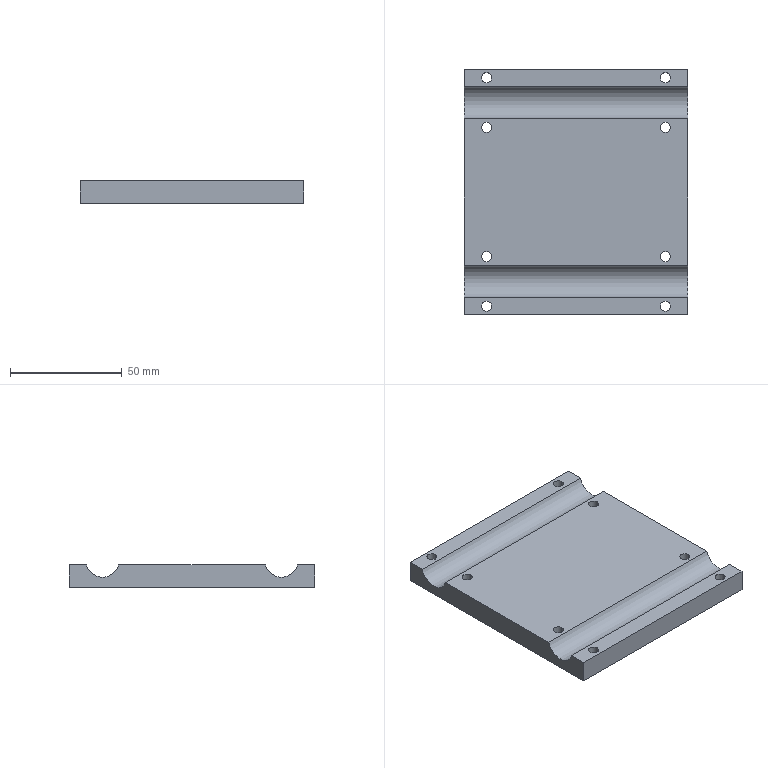Part | STEP file | Cutting module fixing bracket | 1 solid | 26 faces | box 100 x 110 x 10 mm | volume 96984 mm3 | cylinder 18 | plane 8 | commonest cylinder face diameters 4.5 x16 15 x2
STEP:
#1=CARTESIAN_POINT('',(-42.25,68.886,-6.));
#2=VERTEX_POINT('',#1);
#3=CARTESIAN_POINT('',(-37.75,68.886,-6.));
#4=VERTEX_POINT('',#3);
#5=CARTESIAN_POINT('',(-40.,68.886,-6.));
#6=DIRECTION('',(0.,0.,1.));
#7=DIRECTION('',(1.,0.,0.));
#8=AXIS2_PLACEMENT_3D('',#5,#6,#7);
#9=CIRCLE('',#8,2.25);
#10=EDGE_CURVE('',#2,#4,#9,.T.);
#11=ORIENTED_EDGE('',*,*,#10,.F.);
#12=CARTESIAN_POINT('',(-42.25,68.886,4.));
#13=VERTEX_POINT('',#12);
#14=CARTESIAN_POINT('',(-42.25,68.886,-14.));
#15=DIRECTION('',(0.,0.,1.));
#16=VECTOR('',#15,1000.);
#17=LINE('',#14,#16);
#18=EDGE_CURVE('',#2,#13,#17,.T.);
#19=ORIENTED_EDGE('',*,*,#18,.T.);
#20=CARTESIAN_POINT('',(-37.75,68.886,4.));
#21=VERTEX_POINT('',#20);
#22=CARTESIAN_POINT('',(-40.,68.886,4.));
#23=DIRECTION('',(0.,0.,1.));
#24=DIRECTION('',(1.,0.,0.));
#25=AXIS2_PLACEMENT_3D('',#22,#23,#24);
#26=CIRCLE('',#25,2.25);
#27=EDGE_CURVE('',#13,#21,#26,.T.);
#28=ORIENTED_EDGE('',*,*,#27,.T.);
#29=CARTESIAN_POINT('',(-37.75,68.886,-14.));
#30=DIRECTION('',(0.,0.,1.));
#31=VECTOR('',#30,1000.);
#32=LINE('',#29,#31);
#33=EDGE_CURVE('',#4,#21,#32,.T.);
#34=ORIENTED_EDGE('',*,*,#33,.F.);
#35=EDGE_LOOP('',(#11,#19,#28,#34));
#36=FACE_OUTER_BOUND('',#35,.T.);
#37=CARTESIAN_POINT('',(-40.,68.886,-14.));
#38=DIRECTION('',(0.,0.,1.));
#39=DIRECTION('',(1.,0.,0.));
#40=AXIS2_PLACEMENT_3D('',#37,#38,#39);
#41=CYLINDRICAL_SURFACE('',#40,2.25);
#42=ADVANCED_FACE('',(#36),#41,.F.);
#43=CARTESIAN_POINT('',(42.25,68.886,-6.));
#44=VERTEX_POINT('',#43);
#45=CARTESIAN_POINT('',(37.75,68.886,-6.));
#46=VERTEX_POINT('',#45);
#47=CARTESIAN_POINT('',(40.,68.886,-6.));
#48=DIRECTION('',(0.,0.,-1.));
#49=DIRECTION('',(1.,0.,0.));
#50=AXIS2_PLACEMENT_3D('',#47,#48,#49);
#51=CIRCLE('',#50,2.25);
#52=EDGE_CURVE('',#44,#46,#51,.T.);
#53=ORIENTED_EDGE('',*,*,#52,.T.);
#54=CARTESIAN_POINT('',(37.75,68.886,4.));
#55=VERTEX_POINT('',#54);
#56=CARTESIAN_POINT('',(37.75,68.886,-14.));
#57=DIRECTION('',(0.,0.,1.));
#58=VECTOR('',#57,1000.);
#59=LINE('',#56,#58);
#60=EDGE_CURVE('',#46,#55,#59,.T.);
#61=ORIENTED_EDGE('',*,*,#60,.T.);
#62=CARTESIAN_POINT('',(42.25,68.886,4.));
#63=VERTEX_POINT('',#62);
#64=CARTESIAN_POINT('',(40.,68.886,4.));
#65=DIRECTION('',(0.,0.,-1.));
#66=DIRECTION('',(-1.,0.,0.));
#67=AXIS2_PLACEMENT_3D('',#64,#65,#66);
#68=CIRCLE('',#67,2.25);
#69=EDGE_CURVE('',#63,#55,#68,.T.);
#70=ORIENTED_EDGE('',*,*,#69,.F.);
#71=CARTESIAN_POINT('',(42.25,68.886,-14.));
#72=DIRECTION('',(0.,0.,1.));
#73=VECTOR('',#72,1000.);
#74=LINE('',#71,#73);
#75=EDGE_CURVE('',#44,#63,#74,.T.);
#76=ORIENTED_EDGE('',*,*,#75,.F.);
#77=EDGE_LOOP('',(#53,#61,#70,#76));
#78=FACE_OUTER_BOUND('',#77,.T.);
#79=CARTESIAN_POINT('',(40.,68.886,-14.));
#80=DIRECTION('',(0.,0.,1.));
#81=DIRECTION('',(1.,0.,0.));
#82=AXIS2_PLACEMENT_3D('',#79,#80,#81);
#83=CYLINDRICAL_SURFACE('',#82,2.25);
#84=ADVANCED_FACE('',(#78),#83,.F.);
#85=CARTESIAN_POINT('',(37.75,91.114,-6.));
#86=VERTEX_POINT('',#85);
#87=CARTESIAN_POINT('',(42.25,91.114,-6.));
#88=VERTEX_POINT('',#87);
#89=CARTESIAN_POINT('',(40.,91.114,-6.));
#90=DIRECTION('',(0.,0.,1.));
#91=DIRECTION('',(1.,0.,0.));
#92=AXIS2_PLACEMENT_3D('',#89,#90,#91);
#93=CIRCLE('',#92,2.25);
#94=EDGE_CURVE('',#86,#88,#93,.T.);
#95=ORIENTED_EDGE('',*,*,#94,.F.);
#96=CARTESIAN_POINT('',(37.75,91.114,4.));
#97=VERTEX_POINT('',#96);
#98=CARTESIAN_POINT('',(37.75,91.114,-14.));
#99=DIRECTION('',(0.,0.,1.));
#100=VECTOR('',#99,1000.);
#101=LINE('',#98,#100);
#102=EDGE_CURVE('',#86,#97,#101,.T.);
#103=ORIENTED_EDGE('',*,*,#102,.T.);
#104=CARTESIAN_POINT('',(42.25,91.114,4.));
#105=VERTEX_POINT('',#104);
#106=CARTESIAN_POINT('',(40.,91.114,4.));
#107=DIRECTION('',(0.,0.,1.));
#108=DIRECTION('',(-1.,0.,0.));
#109=AXIS2_PLACEMENT_3D('',#106,#107,#108);
#110=CIRCLE('',#109,2.25);
#111=EDGE_CURVE('',#97,#105,#110,.T.);
#112=ORIENTED_EDGE('',*,*,#111,.T.);
#113=CARTESIAN_POINT('',(42.25,91.114,-14.));
#114=DIRECTION('',(0.,0.,1.));
#115=VECTOR('',#114,1000.);
#116=LINE('',#113,#115);
#117=EDGE_CURVE('',#88,#105,#116,.T.);
#118=ORIENTED_EDGE('',*,*,#117,.F.);
#119=EDGE_LOOP('',(#95,#103,#112,#118));
#120=FACE_OUTER_BOUND('',#119,.T.);
#121=CARTESIAN_POINT('',(40.,91.114,-14.));
#122=DIRECTION('',(0.,0.,1.));
#123=DIRECTION('',(1.,0.,0.));
#124=AXIS2_PLACEMENT_3D('',#121,#122,#123);
#125=CYLINDRICAL_SURFACE('',#124,2.25);
#126=ADVANCED_FACE('',(#120),#125,.F.);
#127=CARTESIAN_POINT('',(-37.75,91.114,-6.));
#128=VERTEX_POINT('',#127);
#129=CARTESIAN_POINT('',(-42.25,91.114,-6.));
#130=VERTEX_POINT('',#129);
#131=CARTESIAN_POINT('',(-40.,91.114,-6.));
#132=DIRECTION('',(0.,0.,-1.));
#133=DIRECTION('',(1.,0.,0.));
#134=AXIS2_PLACEMENT_3D('',#131,#132,#133);
#135=CIRCLE('',#134,2.25);
#136=EDGE_CURVE('',#128,#130,#135,.T.);
#137=ORIENTED_EDGE('',*,*,#136,.T.);
#138=CARTESIAN_POINT('',(-42.25,91.114,4.));
#139=VERTEX_POINT('',#138);
#140=CARTESIAN_POINT('',(-42.25,91.114,-14.));
#141=DIRECTION('',(0.,0.,1.));
#142=VECTOR('',#141,1000.);
#143=LINE('',#140,#142);
#144=EDGE_CURVE('',#130,#139,#143,.T.);
#145=ORIENTED_EDGE('',*,*,#144,.T.);
#146=CARTESIAN_POINT('',(-37.75,91.114,4.));
#147=VERTEX_POINT('',#146);
#148=CARTESIAN_POINT('',(-40.,91.114,4.));
#149=DIRECTION('',(0.,0.,-1.));
#150=DIRECTION('',(1.,0.,0.));
#151=AXIS2_PLACEMENT_3D('',#148,#149,#150);
#152=CIRCLE('',#151,2.25);
#153=EDGE_CURVE('',#147,#139,#152,.T.);
#154=ORIENTED_EDGE('',*,*,#153,.F.);
#155=CARTESIAN_POINT('',(-37.75,91.114,-14.));
#156=DIRECTION('',(0.,0.,1.));
#157=VECTOR('',#156,1000.);
#158=LINE('',#155,#157);
#159=EDGE_CURVE('',#128,#147,#158,.T.);
#160=ORIENTED_EDGE('',*,*,#159,.F.);
#161=EDGE_LOOP('',(#137,#145,#154,#160));
#162=FACE_OUTER_BOUND('',#161,.T.);
#163=CARTESIAN_POINT('',(-40.,91.114,-14.));
#164=DIRECTION('',(0.,0.,1.));
#165=DIRECTION('',(1.,0.,0.));
#166=AXIS2_PLACEMENT_3D('',#163,#164,#165);
#167=CYLINDRICAL_SURFACE('',#166,2.25);
#168=ADVANCED_FACE('',(#162),#167,.F.);
#169=CARTESIAN_POINT('',(-37.75,11.114,-6.));
#170=VERTEX_POINT('',#169);
#171=CARTESIAN_POINT('',(-42.25,11.114,-6.));
#172=VERTEX_POINT('',#171);
#173=CARTESIAN_POINT('',(-40.,11.114,-6.));
#174=DIRECTION('',(0.,0.,-1.));
#175=DIRECTION('',(1.,0.,0.));
#176=AXIS2_PLACEMENT_3D('',#173,#174,#175);
#177=CIRCLE('',#176,2.25);
#178=EDGE_CURVE('',#170,#172,#177,.T.);
#179=ORIENTED_EDGE('',*,*,#178,.T.);
#180=CARTESIAN_POINT('',(-42.25,11.114,4.));
#181=VERTEX_POINT('',#180);
#182=CARTESIAN_POINT('',(-42.25,11.114,-14.));
#183=DIRECTION('',(0.,0.,1.));
#184=VECTOR('',#183,1000.);
#185=LINE('',#182,#184);
#186=EDGE_CURVE('',#172,#181,#185,.T.);
#187=ORIENTED_EDGE('',*,*,#186,.T.);
#188=CARTESIAN_POINT('',(-37.75,11.114,4.));
#189=VERTEX_POINT('',#188);
#190=CARTESIAN_POINT('',(-40.,11.114,4.));
#191=DIRECTION('',(0.,0.,-1.));
#192=DIRECTION('',(1.,0.,0.));
#193=AXIS2_PLACEMENT_3D('',#190,#191,#192);
#194=CIRCLE('',#193,2.25);
#195=EDGE_CURVE('',#189,#181,#194,.T.);
#196=ORIENTED_EDGE('',*,*,#195,.F.);
#197=CARTESIAN_POINT('',(-37.75,11.114,-14.));
#198=DIRECTION('',(0.,0.,1.));
#199=VECTOR('',#198,1000.);
#200=LINE('',#197,#199);
#201=EDGE_CURVE('',#170,#189,#200,.T.);
#202=ORIENTED_EDGE('',*,*,#201,.F.);
#203=EDGE_LOOP('',(#179,#187,#196,#202));
#204=FACE_OUTER_BOUND('',#203,.T.);
#205=CARTESIAN_POINT('',(-40.,11.114,-14.));
#206=DIRECTION('',(0.,0.,1.));
#207=DIRECTION('',(1.,0.,0.));
#208=AXIS2_PLACEMENT_3D('',#205,#206,#207);
#209=CYLINDRICAL_SURFACE('',#208,2.25);
#210=ADVANCED_FACE('',(#204),#209,.F.);
#211=CARTESIAN_POINT('',(37.75,11.114,-6.));
#212=VERTEX_POINT('',#211);
#213=CARTESIAN_POINT('',(42.25,11.114,-6.));
#214=VERTEX_POINT('',#213);
#215=CARTESIAN_POINT('',(40.,11.114,-6.));
#216=DIRECTION('',(0.,0.,1.));
#217=DIRECTION('',(1.,0.,0.));
#218=AXIS2_PLACEMENT_3D('',#215,#216,#217);
#219=CIRCLE('',#218,2.25);
#220=EDGE_CURVE('',#212,#214,#219,.T.);
#221=ORIENTED_EDGE('',*,*,#220,.F.);
#222=CARTESIAN_POINT('',(37.75,11.114,4.));
#223=VERTEX_POINT('',#222);
#224=CARTESIAN_POINT('',(37.75,11.114,-14.));
#225=DIRECTION('',(0.,0.,1.));
#226=VECTOR('',#225,1000.);
#227=LINE('',#224,#226);
#228=EDGE_CURVE('',#212,#223,#227,.T.);
#229=ORIENTED_EDGE('',*,*,#228,.T.);
#230=CARTESIAN_POINT('',(42.25,11.114,4.));
#231=VERTEX_POINT('',#230);
#232=CARTESIAN_POINT('',(40.,11.114,4.));
#233=DIRECTION('',(0.,0.,1.));
#234=DIRECTION('',(-1.,0.,0.));
#235=AXIS2_PLACEMENT_3D('',#232,#233,#234);
#236=CIRCLE('',#235,2.25);
#237=EDGE_CURVE('',#223,#231,#236,.T.);
#238=ORIENTED_EDGE('',*,*,#237,.T.);
#239=CARTESIAN_POINT('',(42.25,11.114,-14.));
#240=DIRECTION('',(0.,0.,1.));
#241=VECTOR('',#240,1000.);
#242=LINE('',#239,#241);
#243=EDGE_CURVE('',#214,#231,#242,.T.);
#244=ORIENTED_EDGE('',*,*,#243,.F.);
#245=EDGE_LOOP('',(#221,#229,#238,#244));
#246=FACE_OUTER_BOUND('',#245,.T.);
#247=CARTESIAN_POINT('',(40.,11.114,-14.));
#248=DIRECTION('',(0.,0.,1.));
#249=DIRECTION('',(1.,0.,0.));
#250=AXIS2_PLACEMENT_3D('',#247,#248,#249);
#251=CYLINDRICAL_SURFACE('',#250,2.25);
#252=ADVANCED_FACE('',(#246),#251,.F.);
#253=CARTESIAN_POINT('',(42.25,-11.114,-6.));
#254=VERTEX_POINT('',#253);
#255=CARTESIAN_POINT('',(37.75,-11.114,-6.));
#256=VERTEX_POINT('',#255);
#257=CARTESIAN_POINT('',(40.,-11.114,-6.));
#258=DIRECTION('',(0.,0.,-1.));
#259=DIRECTION('',(1.,0.,0.));
#260=AXIS2_PLACEMENT_3D('',#257,#258,#259);
#261=CIRCLE('',#260,2.25);
#262=EDGE_CURVE('',#254,#256,#261,.T.);
#263=ORIENTED_EDGE('',*,*,#262,.T.);
#264=CARTESIAN_POINT('',(37.75,-11.114,4.));
#265=VERTEX_POINT('',#264);
#266=CARTESIAN_POINT('',(37.75,-11.114,-14.));
#267=DIRECTION('',(0.,0.,1.));
#268=VECTOR('',#267,1000.);
#269=LINE('',#266,#268);
#270=EDGE_CURVE('',#256,#265,#269,.T.);
#271=ORIENTED_EDGE('',*,*,#270,.T.);
#272=CARTESIAN_POINT('',(42.25,-11.114,4.));
#273=VERTEX_POINT('',#272);
#274=CARTESIAN_POINT('',(40.,-11.114,4.));
#275=DIRECTION('',(0.,0.,-1.));
#276=DIRECTION('',(-1.,0.,0.));
#277=AXIS2_PLACEMENT_3D('',#274,#275,#276);
#278=CIRCLE('',#277,2.25);
#279=EDGE_CURVE('',#273,#265,#278,.T.);
#280=ORIENTED_EDGE('',*,*,#279,.F.);
#281=CARTESIAN_POINT('',(42.25,-11.114,-14.));
#282=DIRECTION('',(0.,0.,1.));
#283=VECTOR('',#282,1000.);
#284=LINE('',#281,#283);
#285=EDGE_CURVE('',#254,#273,#284,.T.);
#286=ORIENTED_EDGE('',*,*,#285,.F.);
#287=EDGE_LOOP('',(#263,#271,#280,#286));
#288=FACE_OUTER_BOUND('',#287,.T.);
#289=CARTESIAN_POINT('',(40.,-11.114,-14.));
#290=DIRECTION('',(0.,0.,1.));
#291=DIRECTION('',(1.,0.,0.));
#292=AXIS2_PLACEMENT_3D('',#289,#290,#291);
#293=CYLINDRICAL_SURFACE('',#292,2.25);
#294=ADVANCED_FACE('',(#288),#293,.F.);
#295=CARTESIAN_POINT('',(-42.25,-11.114,-6.));
#296=VERTEX_POINT('',#295);
#297=CARTESIAN_POINT('',(-37.75,-11.114,-6.));
#298=VERTEX_POINT('',#297);
#299=CARTESIAN_POINT('',(-40.,-11.114,-6.));
#300=DIRECTION('',(0.,0.,1.));
#301=DIRECTION('',(1.,0.,0.));
#302=AXIS2_PLACEMENT_3D('',#299,#300,#301);
#303=CIRCLE('',#302,2.25);
#304=EDGE_CURVE('',#296,#298,#303,.T.);
#305=ORIENTED_EDGE('',*,*,#304,.F.);
#306=CARTESIAN_POINT('',(-42.25,-11.114,4.));
#307=VERTEX_POINT('',#306);
#308=CARTESIAN_POINT('',(-42.25,-11.114,-14.));
#309=DIRECTION('',(0.,0.,1.));
#310=VECTOR('',#309,1000.);
#311=LINE('',#308,#310);
#312=EDGE_CURVE('',#296,#307,#311,.T.);
#313=ORIENTED_EDGE('',*,*,#312,.T.);
#314=CARTESIAN_POINT('',(-37.75,-11.114,4.));
#315=VERTEX_POINT('',#314);
#316=CARTESIAN_POINT('',(-40.,-11.114,4.));
#317=DIRECTION('',(0.,0.,1.));
#318=DIRECTION('',(1.,0.,0.));
#319=AXIS2_PLACEMENT_3D('',#316,#317,#318);
#320=CIRCLE('',#319,2.25);
#321=EDGE_CURVE('',#307,#315,#320,.T.);
#322=ORIENTED_EDGE('',*,*,#321,.T.);
#323=CARTESIAN_POINT('',(-37.75,-11.114,-14.));
#324=DIRECTION('',(0.,0.,1.));
#325=VECTOR('',#324,1000.);
#326=LINE('',#323,#325);
#327=EDGE_CURVE('',#298,#315,#326,.T.);
#328=ORIENTED_EDGE('',*,*,#327,.F.);
#329=EDGE_LOOP('',(#305,#313,#322,#328));
#330=FACE_OUTER_BOUND('',#329,.T.);
#331=CARTESIAN_POINT('',(-40.,-11.114,-14.));
#332=DIRECTION('',(0.,0.,1.));
#333=DIRECTION('',(1.,0.,0.));
#334=AXIS2_PLACEMENT_3D('',#331,#332,#333);
#335=CYLINDRICAL_SURFACE('',#334,2.25);
#336=ADVANCED_FACE('',(#330),#335,.F.);
#337=CARTESIAN_POINT('',(-40.,68.886,4.));
#338=DIRECTION('',(0.,0.,1.));
#339=DIRECTION('',(1.,0.,0.));
#340=AXIS2_PLACEMENT_3D('',#337,#338,#339);
#341=CIRCLE('',#340,2.25);
#342=EDGE_CURVE('',#21,#13,#341,.T.);
#343=ORIENTED_EDGE('',*,*,#342,.F.);
#344=ORIENTED_EDGE('',*,*,#27,.F.);
#345=EDGE_LOOP('',(#343,#344));
#346=FACE_BOUND('',#345,.T.);
#347=ORIENTED_EDGE('',*,*,#69,.T.);
#348=CARTESIAN_POINT('',(40.,68.886,4.));
#349=DIRECTION('',(0.,0.,-1.));
#350=DIRECTION('',(-1.,0.,0.));
#351=AXIS2_PLACEMENT_3D('',#348,#349,#350);
#352=CIRCLE('',#351,2.25);
#353=EDGE_CURVE('',#55,#63,#352,.T.);
#354=ORIENTED_EDGE('',*,*,#353,.T.);
#355=EDGE_LOOP('',(#347,#354));
#356=FACE_BOUND('',#355,.T.);
#357=CARTESIAN_POINT('',(40.,11.114,4.));
#358=DIRECTION('',(0.,0.,1.));
#359=DIRECTION('',(-1.,0.,0.));
#360=AXIS2_PLACEMENT_3D('',#357,#358,#359);
#361=CIRCLE('',#360,2.25);
#362=EDGE_CURVE('',#231,#223,#361,.T.);
#363=ORIENTED_EDGE('',*,*,#362,.F.);
#364=ORIENTED_EDGE('',*,*,#237,.F.);
#365=EDGE_LOOP('',(#363,#364));
#366=FACE_BOUND('',#365,.T.);
#367=ORIENTED_EDGE('',*,*,#195,.T.);
#368=CARTESIAN_POINT('',(-40.,11.114,4.));
#369=DIRECTION('',(0.,0.,-1.));
#370=DIRECTION('',(1.,0.,0.));
#371=AXIS2_PLACEMENT_3D('',#368,#369,#370);
#372=CIRCLE('',#371,2.25);
#373=EDGE_CURVE('',#181,#189,#372,.T.);
#374=ORIENTED_EDGE('',*,*,#373,.T.);
#375=EDGE_LOOP('',(#367,#374));
#376=FACE_BOUND('',#375,.T.);
#377=CARTESIAN_POINT('',(-50.,72.772,4.));
#378=VERTEX_POINT('',#377);
#379=CARTESIAN_POINT('',(50.,72.772,4.));
#380=VERTEX_POINT('',#379);
#381=CARTESIAN_POINT('',(66.,72.772,4.));
#382=DIRECTION('',(1.,0.,0.));
#383=VECTOR('',#382,1000.);
#384=LINE('',#381,#383);
#385=EDGE_CURVE('',#378,#380,#384,.T.);
#386=ORIENTED_EDGE('',*,*,#385,.F.);
#387=CARTESIAN_POINT('',(-50.,7.228,4.));
#388=VERTEX_POINT('',#387);
#389=CARTESIAN_POINT('',(-50.,-15.,4.));
#390=DIRECTION('',(0.,-1.,0.));
#391=VECTOR('',#390,1000.);
#392=LINE('',#389,#391);
#393=EDGE_CURVE('',#378,#388,#392,.T.);
#394=ORIENTED_EDGE('',*,*,#393,.T.);
#395=CARTESIAN_POINT('',(50.,7.228,4.));
#396=VERTEX_POINT('',#395);
#397=CARTESIAN_POINT('',(66.,7.228,4.));
#398=DIRECTION('',(-1.,0.,0.));
#399=VECTOR('',#398,1000.);
#400=LINE('',#397,#399);
#401=EDGE_CURVE('',#396,#388,#400,.T.);
#402=ORIENTED_EDGE('',*,*,#401,.F.);
#403=CARTESIAN_POINT('',(50.,15.,4.));
#404=DIRECTION('',(0.,-1.,0.));
#405=VECTOR('',#404,1000.);
#406=LINE('',#403,#405);
#407=EDGE_CURVE('',#380,#396,#406,.T.);
#408=ORIENTED_EDGE('',*,*,#407,.F.);
#409=EDGE_LOOP('',(#386,#394,#402,#408));
#410=FACE_OUTER_BOUND('',#409,.T.);
#411=CARTESIAN_POINT('',(0.,0.,4.));
#412=DIRECTION('',(0.,0.,-1.));
#413=DIRECTION('',(-1.,0.,0.));
#414=AXIS2_PLACEMENT_3D('',#411,#412,#413);
#415=PLANE('',#414);
#416=ADVANCED_FACE('',(#346,#356,#366,#376,#410),#415,.F.);
#417=CARTESIAN_POINT('',(40.,91.114,4.));
#418=DIRECTION('',(0.,0.,1.));
#419=DIRECTION('',(-1.,0.,0.));
#420=AXIS2_PLACEMENT_3D('',#417,#418,#419);
#421=CIRCLE('',#420,2.25);
#422=EDGE_CURVE('',#105,#97,#421,.T.);
#423=ORIENTED_EDGE('',*,*,#422,.F.);
#424=ORIENTED_EDGE('',*,*,#111,.F.);
#425=EDGE_LOOP('',(#423,#424));
#426=FACE_BOUND('',#425,.T.);
#427=ORIENTED_EDGE('',*,*,#153,.T.);
#428=CARTESIAN_POINT('',(-40.,91.114,4.));
#429=DIRECTION('',(0.,0.,-1.));
#430=DIRECTION('',(1.,0.,0.));
#431=AXIS2_PLACEMENT_3D('',#428,#429,#430);
#432=CIRCLE('',#431,2.25);
#433=EDGE_CURVE('',#139,#147,#432,.T.);
#434=ORIENTED_EDGE('',*,*,#433,.T.);
#435=EDGE_LOOP('',(#427,#434));
#436=FACE_BOUND('',#435,.T.);
#437=CARTESIAN_POINT('',(50.,87.228,4.));
#438=VERTEX_POINT('',#437);
#439=CARTESIAN_POINT('',(-50.,87.228,4.));
#440=VERTEX_POINT('',#439);
#441=CARTESIAN_POINT('',(66.,87.228,4.));
#442=DIRECTION('',(-1.,0.,0.));
#443=VECTOR('',#442,1000.);
#444=LINE('',#441,#443);
#445=EDGE_CURVE('',#438,#440,#444,.T.);
#446=ORIENTED_EDGE('',*,*,#445,.F.);
#447=CARTESIAN_POINT('',(50.,95.,4.));
#448=VERTEX_POINT('',#447);
#449=CARTESIAN_POINT('',(50.,15.,4.));
#450=DIRECTION('',(0.,-1.,0.));
#451=VECTOR('',#450,1000.);
#452=LINE('',#449,#451);
#453=EDGE_CURVE('',#448,#438,#452,.T.);
#454=ORIENTED_EDGE('',*,*,#453,.F.);
#455=CARTESIAN_POINT('',(-50.,95.,4.));
#456=VERTEX_POINT('',#455);
#457=CARTESIAN_POINT('',(-50.,95.,4.));
#458=DIRECTION('',(1.,0.,0.));
#459=VECTOR('',#458,1000.);
#460=LINE('',#457,#459);
#461=EDGE_CURVE('',#456,#448,#460,.T.);
#462=ORIENTED_EDGE('',*,*,#461,.F.);
#463=CARTESIAN_POINT('',(-50.,-15.,4.));
#464=DIRECTION('',(0.,-1.,0.));
#465=VECTOR('',#464,1000.);
#466=LINE('',#463,#465);
#467=EDGE_CURVE('',#456,#440,#466,.T.);
#468=ORIENTED_EDGE('',*,*,#467,.T.);
#469=EDGE_LOOP('',(#446,#454,#462,#468));
#470=FACE_OUTER_BOUND('',#469,.T.);
#471=CARTESIAN_POINT('',(0.,0.,4.));
#472=DIRECTION('',(0.,0.,-1.));
#473=DIRECTION('',(-1.,0.,0.));
#474=AXIS2_PLACEMENT_3D('',#471,#472,#473);
#475=PLANE('',#474);
#476=ADVANCED_FACE('',(#426,#436,#470),#475,.F.);
#477=CARTESIAN_POINT('',(50.,80.,6.));
#478=DIRECTION('',(1.,0.,0.));
#479=DIRECTION('',(0.,0.,1.));
#480=AXIS2_PLACEMENT_3D('',#477,#478,#479);
#481=CIRCLE('',#480,7.5);
#482=EDGE_CURVE('',#380,#438,#481,.T.);
#483=ORIENTED_EDGE('',*,*,#482,.F.);
#484=ORIENTED_EDGE('',*,*,#407,.T.);
#485=CARTESIAN_POINT('',(50.,-7.228,4.));
#486=VERTEX_POINT('',#485);
#487=CARTESIAN_POINT('',(50.,0.,6.));
#488=DIRECTION('',(-1.,0.,0.));
#489=DIRECTION('',(0.,0.,1.));
#490=AXIS2_PLACEMENT_3D('',#487,#488,#489);
#491=CIRCLE('',#490,7.5);
#492=EDGE_CURVE('',#396,#486,#491,.T.);
#493=ORIENTED_EDGE('',*,*,#492,.T.);
#494=CARTESIAN_POINT('',(50.,-15.,4.));
#495=VERTEX_POINT('',#494);
#496=CARTESIAN_POINT('',(50.,15.,4.));
#497=DIRECTION('',(0.,-1.,0.));
#498=VECTOR('',#497,1000.);
#499=LINE('',#496,#498);
#500=EDGE_CURVE('',#486,#495,#499,.T.);
#501=ORIENTED_EDGE('',*,*,#500,.T.);
#502=CARTESIAN_POINT('',(50.,-15.,-6.));
#503=VERTEX_POINT('',#502);
#504=CARTESIAN_POINT('',(50.,-15.,6.));
#505=DIRECTION('',(0.,0.,-1.));
#506=VECTOR('',#505,1000.);
#507=LINE('',#504,#506);
#508=EDGE_CURVE('',#495,#503,#507,.T.);
#509=ORIENTED_EDGE('',*,*,#508,.T.);
#510=CARTESIAN_POINT('',(50.,95.,-6.));
#511=VERTEX_POINT('',#510);
#512=CARTESIAN_POINT('',(50.,15.,-6.));
#513=DIRECTION('',(0.,1.,0.));
#514=VECTOR('',#513,1000.);
#515=LINE('',#512,#514);
#516=EDGE_CURVE('',#503,#511,#515,.T.);
#517=ORIENTED_EDGE('',*,*,#516,.T.);
#518=CARTESIAN_POINT('',(50.,95.,4.));
#519=DIRECTION('',(0.,0.,-1.));
#520=VECTOR('',#519,1000.);
#521=LINE('',#518,#520);
#522=EDGE_CURVE('',#448,#511,#521,.T.);
#523=ORIENTED_EDGE('',*,*,#522,.F.);
#524=ORIENTED_EDGE('',*,*,#453,.T.);
#525=EDGE_LOOP('',(#483,#484,#493,#501,#509,#517,#523,#524));
#526=FACE_OUTER_BOUND('',#525,.T.);
#527=CARTESIAN_POINT('',(50.,15.,6.));
#528=DIRECTION('',(-1.,0.,0.));
#529=DIRECTION('',(0.,0.,1.));
#530=AXIS2_PLACEMENT_3D('',#527,#528,#529);
#531=PLANE('',#530);
#532=ADVANCED_FACE('',(#526),#531,.F.);
#533=CARTESIAN_POINT('',(-50.,80.,6.));
#534=DIRECTION('',(1.,0.,0.));
#535=DIRECTION('',(0.,1.,0.));
#536=AXIS2_PLACEMENT_3D('',#533,#534,#535);
#537=CIRCLE('',#536,7.5);
#538=EDGE_CURVE('',#378,#440,#537,.T.);
#539=ORIENTED_EDGE('',*,*,#538,.T.);
#540=ORIENTED_EDGE('',*,*,#467,.F.);
#541=CARTESIAN_POINT('',(-50.,95.,-6.));
#542=VERTEX_POINT('',#541);
#543=CARTESIAN_POINT('',(-50.,95.,-6.));
#544=DIRECTION('',(0.,0.,1.));
#545=VECTOR('',#544,1000.);
#546=LINE('',#543,#545);
#547=EDGE_CURVE('',#542,#456,#546,.T.);
#548=ORIENTED_EDGE('',*,*,#547,.F.);
#549=CARTESIAN_POINT('',(-50.,-15.,-6.));
#550=VERTEX_POINT('',#549);
#551=CARTESIAN_POINT('',(-50.,15.,-6.));
#552=DIRECTION('',(0.,-1.,0.));
#553=VECTOR('',#552,1000.);
#554=LINE('',#551,#553);
#555=EDGE_CURVE('',#542,#550,#554,.T.);
#556=ORIENTED_EDGE('',*,*,#555,.T.);
#557=CARTESIAN_POINT('',(-50.,-15.,4.));
#558=VERTEX_POINT('',#557);
#559=CARTESIAN_POINT('',(-50.,-15.,6.));
#560=DIRECTION('',(0.,0.,-1.));
#561=VECTOR('',#560,1000.);
#562=LINE('',#559,#561);
#563=EDGE_CURVE('',#558,#550,#562,.T.);
#564=ORIENTED_EDGE('',*,*,#563,.F.);
#565=CARTESIAN_POINT('',(-50.,-7.228,4.));
#566=VERTEX_POINT('',#565);
#567=CARTESIAN_POINT('',(-50.,-15.,4.));
#568=DIRECTION('',(0.,-1.,0.));
#569=VECTOR('',#568,1000.);
#570=LINE('',#567,#569);
#571=EDGE_CURVE('',#566,#558,#570,.T.);
#572=ORIENTED_EDGE('',*,*,#571,.F.);
#573=CARTESIAN_POINT('',(-50.,0.,6.));
#574=DIRECTION('',(-1.,0.,0.));
#575=DIRECTION('',(0.,-1.,0.));
#576=AXIS2_PLACEMENT_3D('',#573,#574,#575);
#577=CIRCLE('',#576,7.5);
#578=EDGE_CURVE('',#388,#566,#577,.T.);
#579=ORIENTED_EDGE('',*,*,#578,.F.);
#580=ORIENTED_EDGE('',*,*,#393,.F.);
#581=EDGE_LOOP('',(#539,#540,#548,#556,#564,#572,#579,#580));
#582=FACE_OUTER_BOUND('',#581,.T.);
#583=CARTESIAN_POINT('',(-50.,15.,6.));
#584=DIRECTION('',(1.,0.,0.));
#585=DIRECTION('',(0.,0.,-1.));
#586=AXIS2_PLACEMENT_3D('',#583,#584,#585);
#587=PLANE('',#586);
#588=ADVANCED_FACE('',(#582),#587,.F.);
#589=ORIENTED_EDGE('',*,*,#508,.F.);
#590=CARTESIAN_POINT('',(-50.,-15.,4.));
#591=DIRECTION('',(1.,0.,0.));
#592=VECTOR('',#591,1000.);
#593=LINE('',#590,#592);
#594=EDGE_CURVE('',#558,#495,#593,.T.);
#595=ORIENTED_EDGE('',*,*,#594,.F.);
#596=ORIENTED_EDGE('',*,*,#563,.T.);
#597=CARTESIAN_POINT('',(-50.,-15.,-6.));
#598=DIRECTION('',(1.,0.,0.));
#599=VECTOR('',#598,1000.);
#600=LINE('',#597,#599);
#601=EDGE_CURVE('',#550,#503,#600,.T.);
#602=ORIENTED_EDGE('',*,*,#601,.T.);
#603=EDGE_LOOP('',(#589,#595,#596,#602));
#604=FACE_OUTER_BOUND('',#603,.T.);
#605=CARTESIAN_POINT('',(-50.,-15.,6.));
#606=DIRECTION('',(0.,1.,0.));
#607=DIRECTION('',(0.,0.,1.));
#608=AXIS2_PLACEMENT_3D('',#605,#606,#607);
#609=PLANE('',#608);
#610=ADVANCED_FACE('',(#604),#609,.F.);
#611=CARTESIAN_POINT('',(-40.,68.886,-6.));
#612=DIRECTION('',(0.,0.,1.));
#613=DIRECTION('',(1.,0.,0.));
#614=AXIS2_PLACEMENT_3D('',#611,#612,#613);
#615=CIRCLE('',#614,2.25);
#616=EDGE_CURVE('',#4,#2,#615,.T.);
#617=ORIENTED_EDGE('',*,*,#616,.T.);
#618=ORIENTED_EDGE('',*,*,#10,.T.);
#619=EDGE_LOOP('',(#617,#618));
#620=FACE_BOUND('',#619,.T.);
#621=ORIENTED_EDGE('',*,*,#52,.F.);
#622=CARTESIAN_POINT('',(40.,68.886,-6.));
#623=DIRECTION('',(0.,0.,-1.));
#624=DIRECTION('',(1.,0.,0.));
#625=AXIS2_PLACEMENT_3D('',#622,#623,#624);
#626=CIRCLE('',#625,2.25);
#627=EDGE_CURVE('',#46,#44,#626,.T.);
#628=ORIENTED_EDGE('',*,*,#627,.F.);
#629=EDGE_LOOP('',(#621,#628));
#630=FACE_BOUND('',#629,.T.);
#631=CARTESIAN_POINT('',(40.,91.114,-6.));
#632=DIRECTION('',(0.,0.,1.));
#633=DIRECTION('',(1.,0.,0.));
#634=AXIS2_PLACEMENT_3D('',#631,#632,#633);
#635=CIRCLE('',#634,2.25);
#636=EDGE_CURVE('',#88,#86,#635,.T.);
#637=ORIENTED_EDGE('',*,*,#636,.T.);
#638=ORIENTED_EDGE('',*,*,#94,.T.);
#639=EDGE_LOOP('',(#637,#638));
#640=FACE_BOUND('',#639,.T.);
#641=ORIENTED_EDGE('',*,*,#136,.F.);
#642=CARTESIAN_POINT('',(-40.,91.114,-6.));
#643=DIRECTION('',(0.,0.,-1.));
#644=DIRECTION('',(1.,0.,0.));
#645=AXIS2_PLACEMENT_3D('',#642,#643,#644);
#646=CIRCLE('',#645,2.25);
#647=EDGE_CURVE('',#130,#128,#646,.T.);
#648=ORIENTED_EDGE('',*,*,#647,.F.);
#649=EDGE_LOOP('',(#641,#648));
#650=FACE_BOUND('',#649,.T.);
#651=ORIENTED_EDGE('',*,*,#178,.F.);
#652=CARTESIAN_POINT('',(-40.,11.114,-6.));
#653=DIRECTION('',(0.,0.,-1.));
#654=DIRECTION('',(1.,0.,0.));
#655=AXIS2_PLACEMENT_3D('',#652,#653,#654);
#656=CIRCLE('',#655,2.25);
#657=EDGE_CURVE('',#172,#170,#656,.T.);
#658=ORIENTED_EDGE('',*,*,#657,.F.);
#659=EDGE_LOOP('',(#651,#658));
#660=FACE_BOUND('',#659,.T.);
#661=CARTESIAN_POINT('',(40.,11.114,-6.));
#662=DIRECTION('',(0.,0.,1.));
#663=DIRECTION('',(1.,0.,0.));
#664=AXIS2_PLACEMENT_3D('',#661,#662,#663);
#665=CIRCLE('',#664,2.25);
#666=EDGE_CURVE('',#214,#212,#665,.T.);
#667=ORIENTED_EDGE('',*,*,#666,.T.);
#668=ORIENTED_EDGE('',*,*,#220,.T.);
#669=EDGE_LOOP('',(#667,#668));
#670=FACE_BOUND('',#669,.T.);
#671=ORIENTED_EDGE('',*,*,#262,.F.);
#672=CARTESIAN_POINT('',(40.,-11.114,-6.));
#673=DIRECTION('',(0.,0.,-1.));
#674=DIRECTION('',(1.,0.,0.));
#675=AXIS2_PLACEMENT_3D('',#672,#673,#674);
#676=CIRCLE('',#675,2.25);
#677=EDGE_CURVE('',#256,#254,#676,.T.);
#678=ORIENTED_EDGE('',*,*,#677,.F.);
#679=EDGE_LOOP('',(#671,#678));
#680=FACE_BOUND('',#679,.T.);
#681=CARTESIAN_POINT('',(-40.,-11.114,-6.));
#682=DIRECTION('',(0.,0.,1.));
#683=DIRECTION('',(1.,0.,0.));
#684=AXIS2_PLACEMENT_3D('',#681,#682,#683);
#685=CIRCLE('',#684,2.25);
#686=EDGE_CURVE('',#298,#296,#685,.T.);
#687=ORIENTED_EDGE('',*,*,#686,.T.);
#688=ORIENTED_EDGE('',*,*,#304,.T.);
#689=EDGE_LOOP('',(#687,#688));
#690=FACE_BOUND('',#689,.T.);
#691=ORIENTED_EDGE('',*,*,#516,.F.);
#692=ORIENTED_EDGE('',*,*,#601,.F.);
#693=ORIENTED_EDGE('',*,*,#555,.F.);
#694=CARTESIAN_POINT('',(50.,95.,-6.));
#695=DIRECTION('',(-1.,0.,0.));
#696=VECTOR('',#695,1000.);
#697=LINE('',#694,#696);
#698=EDGE_CURVE('',#511,#542,#697,.T.);
#699=ORIENTED_EDGE('',*,*,#698,.F.);
#700=EDGE_LOOP('',(#691,#692,#693,#699));
#701=FACE_OUTER_BOUND('',#700,.T.);
#702=CARTESIAN_POINT('',(0.,0.,-6.));
#703=DIRECTION('',(0.,0.,1.));
#704=DIRECTION('',(1.,0.,0.));
#705=AXIS2_PLACEMENT_3D('',#702,#703,#704);
#706=PLANE('',#705);
#707=ADVANCED_FACE('',(#620,#630,#640,#650,#660,#670,#680,#690,#701),#706,.F.);
#708=ORIENTED_EDGE('',*,*,#578,.T.);
#709=CARTESIAN_POINT('',(66.,-7.228,4.));
#710=DIRECTION('',(1.,0.,0.));
#711=VECTOR('',#710,1000.);
#712=LINE('',#709,#711);
#713=EDGE_CURVE('',#566,#486,#712,.T.);
#714=ORIENTED_EDGE('',*,*,#713,.T.);
#715=ORIENTED_EDGE('',*,*,#492,.F.);
#716=ORIENTED_EDGE('',*,*,#401,.T.);
#717=EDGE_LOOP('',(#708,#714,#715,#716));
#718=FACE_OUTER_BOUND('',#717,.T.);
#719=CARTESIAN_POINT('',(66.,0.,6.));
#720=DIRECTION('',(-1.,0.,0.));
#721=DIRECTION('',(0.,-1.,0.));
#722=AXIS2_PLACEMENT_3D('',#719,#720,#721);
#723=CYLINDRICAL_SURFACE('',#722,7.5);
#724=ADVANCED_FACE('',(#718),#723,.F.);
#725=ORIENTED_EDGE('',*,*,#279,.T.);
#726=CARTESIAN_POINT('',(40.,-11.114,4.));
#727=DIRECTION('',(0.,0.,-1.));
#728=DIRECTION('',(-1.,0.,0.));
#729=AXIS2_PLACEMENT_3D('',#726,#727,#728);
#730=CIRCLE('',#729,2.25);
#731=EDGE_CURVE('',#265,#273,#730,.T.);
#732=ORIENTED_EDGE('',*,*,#731,.T.);
#733=EDGE_LOOP('',(#725,#732));
#734=FACE_BOUND('',#733,.T.);
#735=CARTESIAN_POINT('',(-40.,-11.114,4.));
#736=DIRECTION('',(0.,0.,1.));
#737=DIRECTION('',(1.,0.,0.));
#738=AXIS2_PLACEMENT_3D('',#735,#736,#737);
#739=CIRCLE('',#738,2.25);
#740=EDGE_CURVE('',#315,#307,#739,.T.);
#741=ORIENTED_EDGE('',*,*,#740,.F.);
#742=ORIENTED_EDGE('',*,*,#321,.F.);
#743=EDGE_LOOP('',(#741,#742));
#744=FACE_BOUND('',#743,.T.);
#745=ORIENTED_EDGE('',*,*,#713,.F.);
#746=ORIENTED_EDGE('',*,*,#571,.T.);
#747=ORIENTED_EDGE('',*,*,#594,.T.);
#748=ORIENTED_EDGE('',*,*,#500,.F.);
#749=EDGE_LOOP('',(#745,#746,#747,#748));
#750=FACE_OUTER_BOUND('',#749,.T.);
#751=CARTESIAN_POINT('',(0.,0.,4.));
#752=DIRECTION('',(0.,0.,-1.));
#753=DIRECTION('',(-1.,0.,0.));
#754=AXIS2_PLACEMENT_3D('',#751,#752,#753);
#755=PLANE('',#754);
#756=ADVANCED_FACE('',(#734,#744,#750),#755,.F.);
#757=ORIENTED_EDGE('',*,*,#312,.F.);
#758=ORIENTED_EDGE('',*,*,#686,.F.);
#759=ORIENTED_EDGE('',*,*,#327,.T.);
#760=ORIENTED_EDGE('',*,*,#740,.T.);
#761=EDGE_LOOP('',(#757,#758,#759,#760));
#762=FACE_OUTER_BOUND('',#761,.T.);
#763=CARTESIAN_POINT('',(-40.,-11.114,-14.));
#764=DIRECTION('',(0.,0.,1.));
#765=DIRECTION('',(1.,0.,0.));
#766=AXIS2_PLACEMENT_3D('',#763,#764,#765);
#767=CYLINDRICAL_SURFACE('',#766,2.25);
#768=ADVANCED_FACE('',(#762),#767,.F.);
#769=ORIENTED_EDGE('',*,*,#270,.F.);
#770=ORIENTED_EDGE('',*,*,#677,.T.);
#771=ORIENTED_EDGE('',*,*,#285,.T.);
#772=ORIENTED_EDGE('',*,*,#731,.F.);
#773=EDGE_LOOP('',(#769,#770,#771,#772));
#774=FACE_OUTER_BOUND('',#773,.T.);
#775=CARTESIAN_POINT('',(40.,-11.114,-14.));
#776=DIRECTION('',(0.,0.,1.));
#777=DIRECTION('',(1.,0.,0.));
#778=AXIS2_PLACEMENT_3D('',#775,#776,#777);
#779=CYLINDRICAL_SURFACE('',#778,2.25);
#780=ADVANCED_FACE('',(#774),#779,.F.);
#781=ORIENTED_EDGE('',*,*,#228,.F.);
#782=ORIENTED_EDGE('',*,*,#666,.F.);
#783=ORIENTED_EDGE('',*,*,#243,.T.);
#784=ORIENTED_EDGE('',*,*,#362,.T.);
#785=EDGE_LOOP('',(#781,#782,#783,#784));
#786=FACE_OUTER_BOUND('',#785,.T.);
#787=CARTESIAN_POINT('',(40.,11.114,-14.));
#788=DIRECTION('',(0.,0.,1.));
#789=DIRECTION('',(1.,0.,0.));
#790=AXIS2_PLACEMENT_3D('',#787,#788,#789);
#791=CYLINDRICAL_SURFACE('',#790,2.25);
#792=ADVANCED_FACE('',(#786),#791,.F.);
#793=ORIENTED_EDGE('',*,*,#186,.F.);
#794=ORIENTED_EDGE('',*,*,#657,.T.);
#795=ORIENTED_EDGE('',*,*,#201,.T.);
#796=ORIENTED_EDGE('',*,*,#373,.F.);
#797=EDGE_LOOP('',(#793,#794,#795,#796));
#798=FACE_OUTER_BOUND('',#797,.T.);
#799=CARTESIAN_POINT('',(-40.,11.114,-14.));
#800=DIRECTION('',(0.,0.,1.));
#801=DIRECTION('',(1.,0.,0.));
#802=AXIS2_PLACEMENT_3D('',#799,#800,#801);
#803=CYLINDRICAL_SURFACE('',#802,2.25);
#804=ADVANCED_FACE('',(#798),#803,.F.);
#805=ORIENTED_EDGE('',*,*,#698,.T.);
#806=ORIENTED_EDGE('',*,*,#547,.T.);
#807=ORIENTED_EDGE('',*,*,#461,.T.);
#808=ORIENTED_EDGE('',*,*,#522,.T.);
#809=EDGE_LOOP('',(#805,#806,#807,#808));
#810=FACE_OUTER_BOUND('',#809,.T.);
#811=CARTESIAN_POINT('',(0.,95.,0.));
#812=DIRECTION('',(0.,1.,0.));
#813=DIRECTION('',(0.,0.,1.));
#814=AXIS2_PLACEMENT_3D('',#811,#812,#813);
#815=PLANE('',#814);
#816=ADVANCED_FACE('',(#810),#815,.T.);
#817=ORIENTED_EDGE('',*,*,#385,.T.);
#818=ORIENTED_EDGE('',*,*,#482,.T.);
#819=ORIENTED_EDGE('',*,*,#445,.T.);
#820=ORIENTED_EDGE('',*,*,#538,.F.);
#821=EDGE_LOOP('',(#817,#818,#819,#820));
#822=FACE_OUTER_BOUND('',#821,.T.);
#823=CARTESIAN_POINT('',(66.,80.,6.));
#824=DIRECTION('',(-1.,0.,0.));
#825=DIRECTION('',(0.,-1.,0.));
#826=AXIS2_PLACEMENT_3D('',#823,#824,#825);
#827=CYLINDRICAL_SURFACE('',#826,7.5);
#828=ADVANCED_FACE('',(#822),#827,.F.);
#829=ORIENTED_EDGE('',*,*,#144,.F.);
#830=ORIENTED_EDGE('',*,*,#647,.T.);
#831=ORIENTED_EDGE('',*,*,#159,.T.);
#832=ORIENTED_EDGE('',*,*,#433,.F.);
#833=EDGE_LOOP('',(#829,#830,#831,#832));
#834=FACE_OUTER_BOUND('',#833,.T.);
#835=CARTESIAN_POINT('',(-40.,91.114,-14.));
#836=DIRECTION('',(0.,0.,1.));
#837=DIRECTION('',(1.,0.,0.));
#838=AXIS2_PLACEMENT_3D('',#835,#836,#837);
#839=CYLINDRICAL_SURFACE('',#838,2.25);
#840=ADVANCED_FACE('',(#834),#839,.F.);
#841=ORIENTED_EDGE('',*,*,#102,.F.);
#842=ORIENTED_EDGE('',*,*,#636,.F.);
#843=ORIENTED_EDGE('',*,*,#117,.T.);
#844=ORIENTED_EDGE('',*,*,#422,.T.);
#845=EDGE_LOOP('',(#841,#842,#843,#844));
#846=FACE_OUTER_BOUND('',#845,.T.);
#847=CARTESIAN_POINT('',(40.,91.114,-14.));
#848=DIRECTION('',(0.,0.,1.));
#849=DIRECTION('',(1.,0.,0.));
#850=AXIS2_PLACEMENT_3D('',#847,#848,#849);
#851=CYLINDRICAL_SURFACE('',#850,2.25);
#852=ADVANCED_FACE('',(#846),#851,.F.);
#853=ORIENTED_EDGE('',*,*,#60,.F.);
#854=ORIENTED_EDGE('',*,*,#627,.T.);
#855=ORIENTED_EDGE('',*,*,#75,.T.);
#856=ORIENTED_EDGE('',*,*,#353,.F.);
#857=EDGE_LOOP('',(#853,#854,#855,#856));
#858=FACE_OUTER_BOUND('',#857,.T.);
#859=CARTESIAN_POINT('',(40.,68.886,-14.));
#860=DIRECTION('',(0.,0.,1.));
#861=DIRECTION('',(1.,0.,0.));
#862=AXIS2_PLACEMENT_3D('',#859,#860,#861);
#863=CYLINDRICAL_SURFACE('',#862,2.25);
#864=ADVANCED_FACE('',(#858),#863,.F.);
#865=ORIENTED_EDGE('',*,*,#18,.F.);
#866=ORIENTED_EDGE('',*,*,#616,.F.);
#867=ORIENTED_EDGE('',*,*,#33,.T.);
#868=ORIENTED_EDGE('',*,*,#342,.T.);
#869=EDGE_LOOP('',(#865,#866,#867,#868));
#870=FACE_OUTER_BOUND('',#869,.T.);
#871=CARTESIAN_POINT('',(-40.,68.886,-14.));
#872=DIRECTION('',(0.,0.,1.));
#873=DIRECTION('',(1.,0.,0.));
#874=AXIS2_PLACEMENT_3D('',#871,#872,#873);
#875=CYLINDRICAL_SURFACE('',#874,2.25);
#876=ADVANCED_FACE('',(#870),#875,.F.);
#877=CLOSED_SHELL('',(#42,#84,#126,#168,#210,#252,#294,#336,#416,#476,#532,#588,#610,#707,#724,#756,#768,#780,#792,#804,#816,#828,#840,#852,#864,#876));
#878=MANIFOLD_SOLID_BREP('',#877);
#879=CARTESIAN_POINT('',(0.,0.,0.));
#880=DIRECTION('',(0.,0.,1.));
#881=DIRECTION('',(1.,0.,0.));
#882=AXIS2_PLACEMENT_3D('',#879,#880,#881);
#883=(LENGTH_UNIT()NAMED_UNIT(*)SI_UNIT(.MILLI.,.METRE.));
#884=UNCERTAINTY_MEASURE_WITH_UNIT(LENGTH_MEASURE(0.00001),#883,'','');
#885=(NAMED_UNIT(*)PLANE_ANGLE_UNIT()SI_UNIT($,.RADIAN.));
#886=(NAMED_UNIT(*)SI_UNIT($,.STERADIAN.)SOLID_ANGLE_UNIT());
#887=(GEOMETRIC_REPRESENTATION_CONTEXT(3)GLOBAL_UNCERTAINTY_ASSIGNED_CONTEXT((#884))GLOBAL_UNIT_ASSIGNED_CONTEXT((#883,#885,#886))REPRESENTATION_CONTEXT('',''));
#888=ADVANCED_BREP_SHAPE_REPRESENTATION('',(#878,#882),#887);